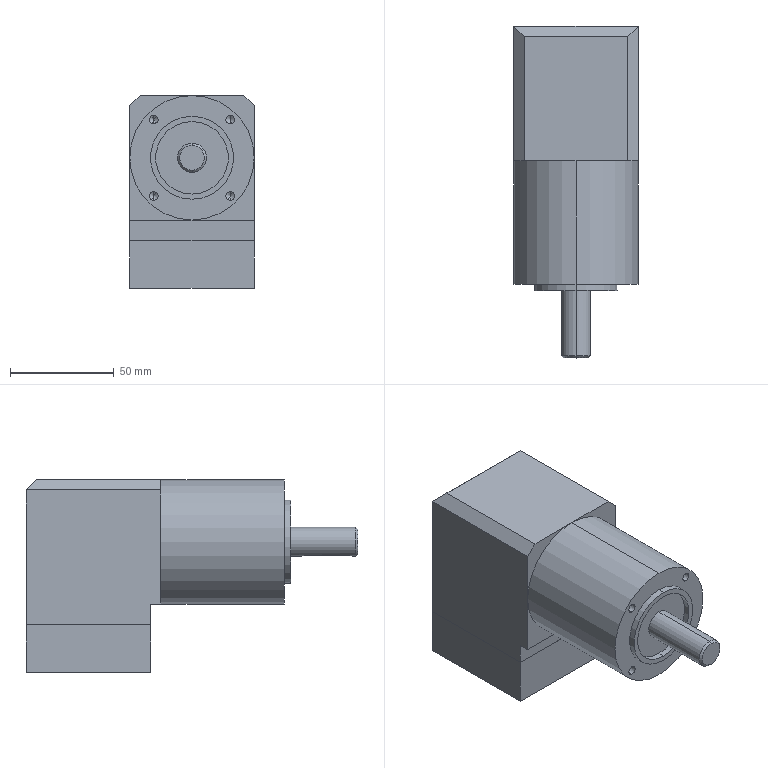Part | STEP file | Right-Angle Reducer WPLE60-100 | 1 solid | 79 faces | box 60.05 x 160.025 x 93 mm | volume 504170 mm3 | cylinder 32 | plane 29 | cone 18 | commonest cylinder face diameters 4.2 x16 14 x4 35 x4 5 x2 40 x2 50 x2